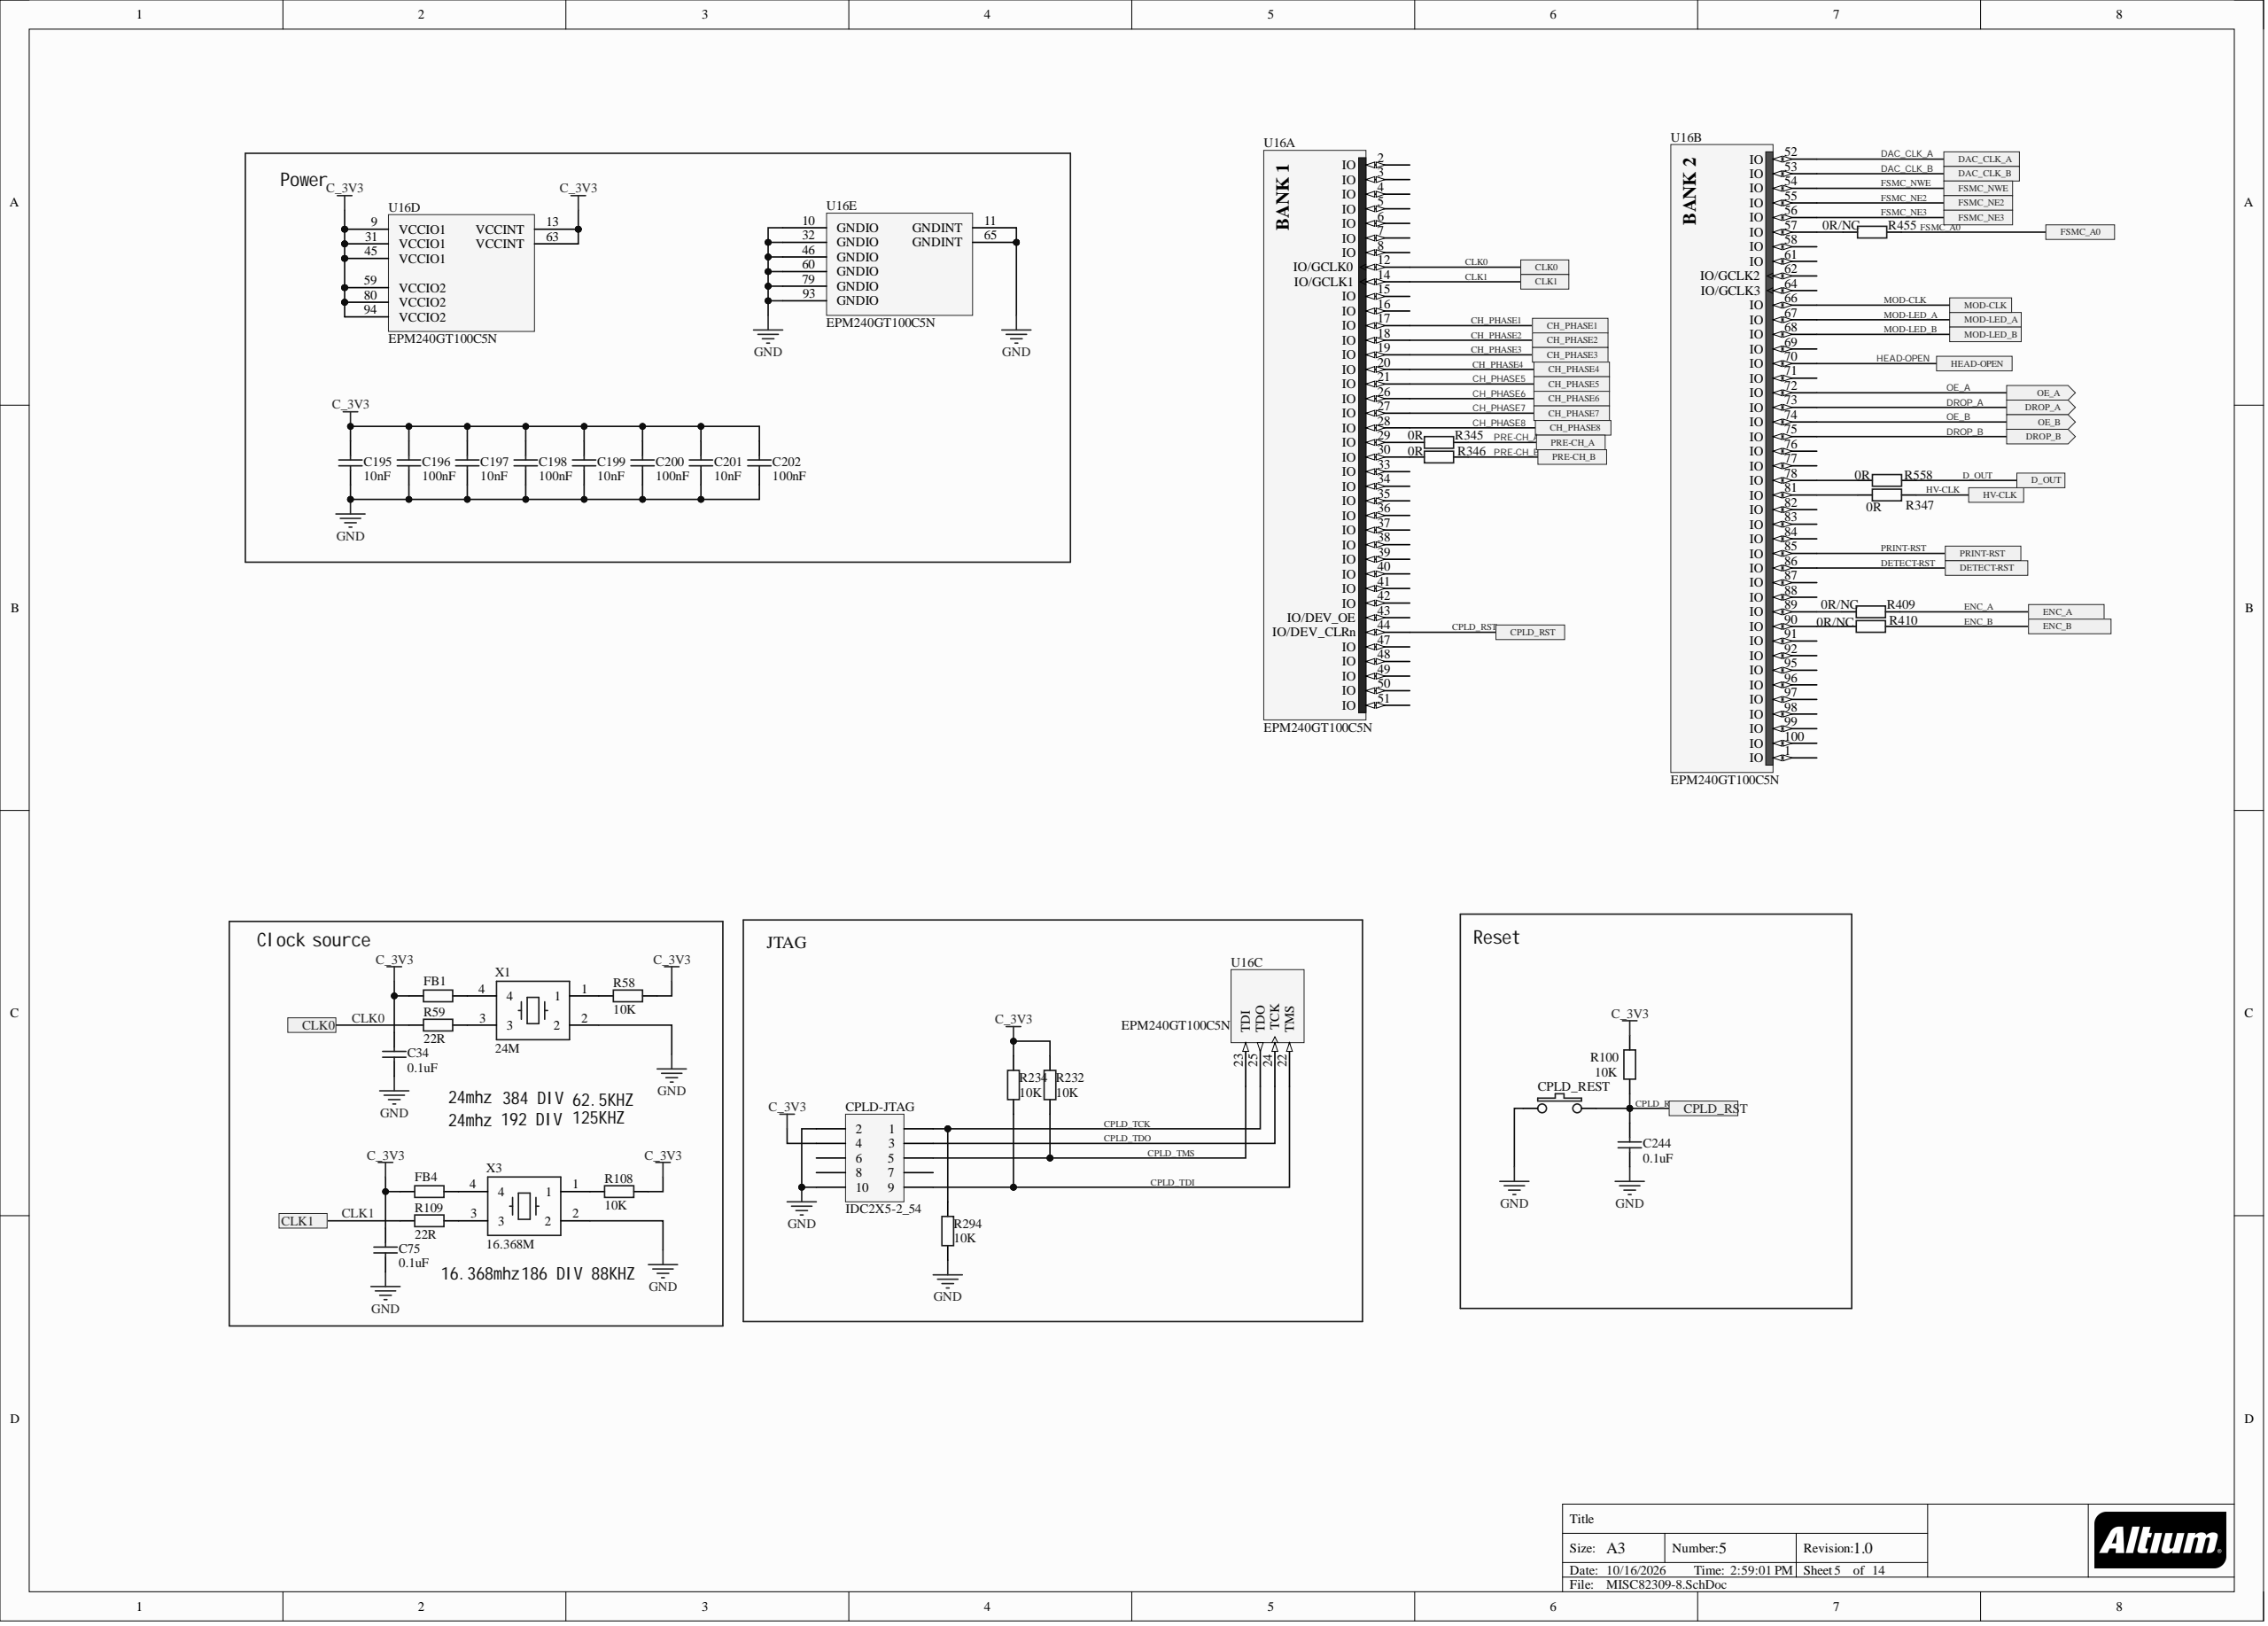Circuit board | Altium Designer | 747 parts | 576 nets | one sheet of the schematic
Parts on this sheet (reference | value | footprint):
C34 | 0.1uF | C0603
C75 | 0.1uF | C0603
C195 | 10nF | C0805
C196 | 100nF | C0805
C197 | 10nF | C0805
C198 | 100nF | C0805
C199 | 10nF | C0805
C200 | 100nF | C0805
C201 | 10nF | C0805
C202 | 100nF | C0805
C244 | 0.1uF | C0603
CPLD-JTAG | IDC2X5-2_54 | IDC2X5-2_54
CPLD_REST | SW | SW-6X3X2.5
FB1 | 60 | SMD1206-L
FB4 | 60 | SMD1206-L
R58 | 10K | R0603
R59 | 22R | R0603
R100 | 10K | R0603
R108 | 10K | R0603
R109 | 22R | R0603
R232 | 10K | R0603
R234 | 10K | R0603
R294 | 10K | R0603
R345 | 0R | RES_0603
R346 | 0R | RES_0603
R347 | 0R | RES_0603
R409 | 0R/NC | RES_0603
R410 | 0R/NC | RES_0603
R455 | 0R/NC | RES_0603
U16 | EPM240GT100C5N | TQFP100_N
X1 | 24M | SMD5032
X3 | 16.368M | SMD5032
Nets of these parts (net: part-pin ...):
PRINT-RST: U16-85
PRE-CH_B: R346-2
PRE-CH_A: R345-2
OE_B: U16-74
OE_A: U16-72
NetR455_1: R455-1 U16-57
NetR410_1: R410-1 U16-90
NetR409_1: R409-1 U16-89
NetR347_1: R347-1 U16-81
NetR346_1: R346-1 U16-30
NetR345_1: R345-1 U16-29
NetR109_2: R109-2 X3-3
NetR108_1: R108-1 X3-1
NetR59_2: R59-2 X1-3
NetR58_1: R58-1 X1-1
NetFB4_2: FB4-2 X3-4
NetFB1_2: FB1-2 X1-4
MOD-LED_B: U16-68
MOD-LED_A: U16-67
MOD-CLK: U16-66
HV-CLK: R347-2
HEAD-OPEN: U16-70
GND: C34-1 C75-1 C195-1 C196-1 C197-1 C198-1 C199-1 C200-1 C201-1 C202-1 C244-1 CPLD-JTAG-2 CPLD-JTAG-10 CPLD_REST-1 R294-1 X1-2 X3-2 U16-10 U16-11 U16-32 U16-46 U16-60 U16-65 U16-79 U16-93
FSMC_NWE: U16-54
FSMC_NE3: U16-56
FSMC_NE2: U16-55
FSMC_A0: R455-2
ENC_B: R410-2
ENC_A: R409-2
DROP_B: U16-75
DROP_A: U16-73
DETECT-RST: U16-86
DAC_CLK_B: U16-53
DAC_CLK_A: U16-52
CPLD_TMS: CPLD-JTAG-5 R232-1 U16-23
CPLD_TDO: CPLD-JTAG-3 U16-24
CPLD_TDI: CPLD-JTAG-9 R234-1 U16-22
CPLD_TCK: CPLD-JTAG-1 R294-2 U16-25
CPLD_RST: C244-2 CPLD_REST-2 R100-2 U16-44
CLK1: R109-1 U16-14
CLK0: R59-1 U16-12
CH_PHASE8: U16-28
CH_PHASE7: U16-27
CH_PHASE6: U16-26
CH_PHASE5: U16-21
CH_PHASE4: U16-20
CH_PHASE3: U16-19
CH_PHASE2: U16-18
CH_PHASE1: U16-17
C_3V3: C34-2 C75-2 C195-2 C196-2 C197-2 C198-2 C199-2 C200-2 C201-2 C202-2 CPLD-JTAG-4 FB1-1 FB4-1 R58-2 R100-1 R108-2 R232-2 R234-2 U16-9 U16-13 U16-31 U16-45 U16-59 U16-63 U16-80 U16-94